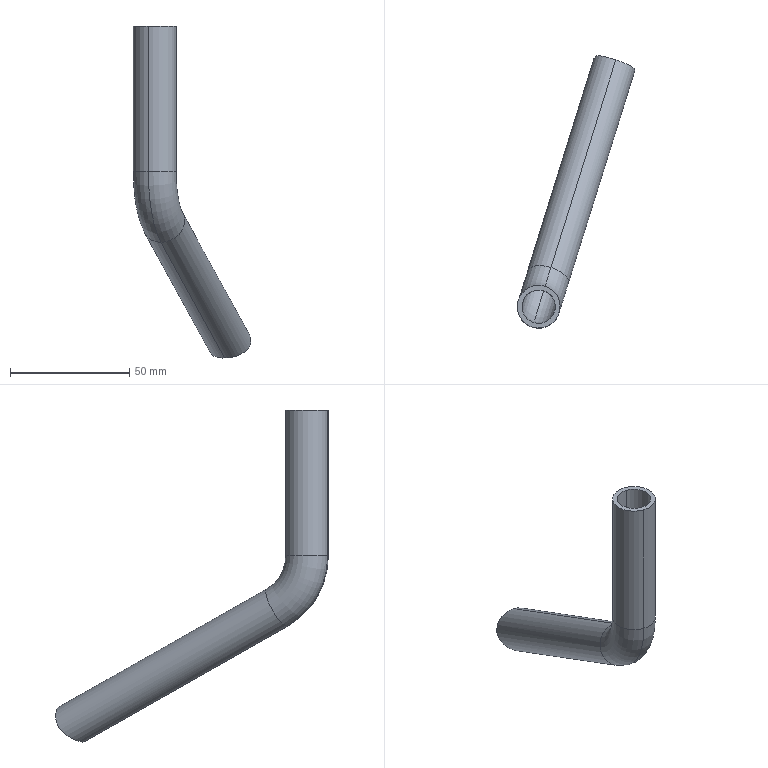Part | SolidWorks | features BaseBody 1 | 1 solid | 17 faces | box 49.357 x 114.676 x 139.496 mm | volume 19339 mm3 | cylinder 8 | spline 4 | torus 4 | plane 1 | commonest cylinder face diameters 14 x4 18 x4
STEP:
#1=CARTESIAN_POINT('',(32.452,94.694,-127.45));
#2=VERTEX_POINT('',#1);
#3=CARTESIAN_POINT('',(32.101,102.969,-116.416));
#4=VERTEX_POINT('',#3);
#5=CARTESIAN_POINT('',(32.452,94.694,-127.45));
#6=CARTESIAN_POINT('',(32.716,94.736,-127.396));
#7=CARTESIAN_POINT('',(33.249,94.856,-127.273));
#8=CARTESIAN_POINT('',(34.046,95.146,-127.049));
#9=CARTESIAN_POINT('',(34.836,95.548,-126.779));
#10=CARTESIAN_POINT('',(35.597,96.049,-126.464));
#11=CARTESIAN_POINT('',(36.325,96.649,-126.09));
#12=CARTESIAN_POINT('',(36.956,97.286,-125.671));
#13=CARTESIAN_POINT('',(37.437,97.864,-125.25));
#14=CARTESIAN_POINT('',(37.805,98.383,-124.818));
#15=CARTESIAN_POINT('',(38.075,98.836,-124.376));
#16=CARTESIAN_POINT('',(38.261,99.224,-123.927));
#17=CARTESIAN_POINT('',(38.377,99.559,-123.464));
#18=CARTESIAN_POINT('',(38.433,99.854,-122.972));
#19=CARTESIAN_POINT('',(38.426,100.121,-122.437));
#20=CARTESIAN_POINT('',(38.349,100.367,-121.842));
#21=CARTESIAN_POINT('',(38.186,100.594,-121.183));
#22=CARTESIAN_POINT('',(37.924,100.807,-120.472));
#23=CARTESIAN_POINT('',(37.548,101.015,-119.722));
#24=CARTESIAN_POINT('',(37.048,101.229,-118.965));
#25=CARTESIAN_POINT('',(36.455,101.448,-118.273));
#26=CARTESIAN_POINT('',(35.795,101.677,-117.678));
#27=CARTESIAN_POINT('',(35.106,101.913,-117.204));
#28=CARTESIAN_POINT('',(34.377,102.163,-116.834));
#29=CARTESIAN_POINT('',(33.621,102.427,-116.575));
#30=CARTESIAN_POINT('',(32.859,102.697,-116.432));
#31=CARTESIAN_POINT('',(32.352,102.878,-116.409));
#32=CARTESIAN_POINT('',(32.101,102.969,-116.416));
#33=B_SPLINE_CURVE_WITH_KNOTS('',3,(#5,#6,#7,#8,#9,#10,#11,#12,#13,#14,#15,#16,#17,#18,#19,#20,#21,#22,#23,#24,#25,#26,#27,#28,#29,#30,#31,#32),.UNSPECIFIED.,.F.,.F.,(4,1,1,1,1,1,1,1,1,1,1,1,1,1,1,1,1,1,1,1,1,1,1,1,1,4),(0.,0.04,0.08,0.12,0.16,0.2,0.24,0.28,0.32,0.36,0.4,0.44,0.48,0.52,0.56,0.6,0.64,0.68,0.72,0.76,0.8,0.84,0.88,0.92,0.96,1.),.UNSPECIFIED.);
#34=EDGE_CURVE('',#2,#4,#33,.T.);
#35=ORIENTED_EDGE('',*,*,#34,.F.);
#36=CARTESIAN_POINT('',(29.565,94.835,-127.721));
#37=VERTEX_POINT('',#36);
#38=CARTESIAN_POINT('',(29.565,94.835,-127.721));
#39=CARTESIAN_POINT('',(29.743,94.761,-127.712));
#40=CARTESIAN_POINT('',(30.105,94.639,-127.689));
#41=CARTESIAN_POINT('',(30.66,94.532,-127.645));
#42=CARTESIAN_POINT('',(31.232,94.5,-127.59));
#43=CARTESIAN_POINT('',(31.828,94.546,-127.526));
#44=CARTESIAN_POINT('',(32.242,94.635,-127.477));
#45=CARTESIAN_POINT('',(32.452,94.694,-127.45));
#46=B_SPLINE_CURVE_WITH_KNOTS('',3,(#38,#39,#40,#41,#42,#43,#44,#45),.UNSPECIFIED.,.F.,.F.,(4,1,1,1,1,4),(0.,0.2,0.4,0.6,0.8,1.),.UNSPECIFIED.);
#47=EDGE_CURVE('',#37,#2,#46,.T.);
#48=ORIENTED_EDGE('',*,*,#47,.F.);
#49=CARTESIAN_POINT('',(2.9,9.302,-79.129));
#50=VERTEX_POINT('',#49);
#51=CARTESIAN_POINT('',(29.565,94.835,-127.721));
#52=DIRECTION('',(-0.2616,-0.8392,0.4768));
#53=VECTOR('',#52,1000.);
#54=LINE('',#51,#53);
#55=EDGE_CURVE('',#37,#50,#54,.T.);
#56=ORIENTED_EDGE('',*,*,#55,.T.);
#57=CARTESIAN_POINT('',(4.887,15.674,-66.823));
#58=VERTEX_POINT('',#57);
#59=CARTESIAN_POINT('',(3.893,12.488,-72.976));
#60=DIRECTION('',(-0.2616,-0.8392,0.4768));
#61=DIRECTION('',(-0.1419,-0.4552,-0.879));
#62=AXIS2_PLACEMENT_3D('',#59,#60,#61);
#63=CIRCLE('',#62,7.);
#64=EDGE_CURVE('',#50,#58,#63,.T.);
#65=ORIENTED_EDGE('',*,*,#64,.T.);
#66=CARTESIAN_POINT('',(32.101,102.969,-116.416));
#67=DIRECTION('',(-0.2616,-0.8392,0.4768));
#68=VECTOR('',#67,1000.);
#69=LINE('',#66,#68);
#70=EDGE_CURVE('',#4,#58,#69,.T.);
#71=ORIENTED_EDGE('',*,*,#70,.F.);
#72=EDGE_LOOP('',(#35,#48,#56,#65,#71));
#73=FACE_OUTER_BOUND('',#72,.T.);
#74=CARTESIAN_POINT('',(3.893,12.488,-72.976));
#75=DIRECTION('',(0.2616,0.8392,-0.4768));
#76=DIRECTION('',(-0.1419,-0.4552,-0.879));
#77=AXIS2_PLACEMENT_3D('',#74,#75,#76);
#78=CYLINDRICAL_SURFACE('',#77,7.);
#79=ADVANCED_FACE('',(#73),#78,.F.);
#80=CARTESIAN_POINT('',(3.893,12.488,-72.976));
#81=DIRECTION('',(-0.2616,-0.8392,0.4768));
#82=DIRECTION('',(0.1419,0.4552,0.879));
#83=AXIS2_PLACEMENT_3D('',#80,#81,#82);
#84=CIRCLE('',#83,7.);
#85=EDGE_CURVE('',#58,#50,#84,.T.);
#86=ORIENTED_EDGE('',*,*,#85,.T.);
#87=ORIENTED_EDGE('',*,*,#55,.F.);
#88=CARTESIAN_POINT('',(28.332,95.591,-127.753));
#89=VERTEX_POINT('',#88);
#90=CARTESIAN_POINT('',(28.332,95.591,-127.753));
#91=CARTESIAN_POINT('',(28.466,95.48,-127.754));
#92=CARTESIAN_POINT('',(28.736,95.275,-127.752));
#93=CARTESIAN_POINT('',(29.146,95.025,-127.741));
#94=CARTESIAN_POINT('',(29.425,94.892,-127.728));
#95=CARTESIAN_POINT('',(29.565,94.835,-127.721));
#96=B_SPLINE_CURVE_WITH_KNOTS('',3,(#90,#91,#92,#93,#94,#95),.UNSPECIFIED.,.F.,.F.,(4,1,1,4),(0.,0.3333,0.6667,1.),.UNSPECIFIED.);
#97=EDGE_CURVE('',#89,#37,#96,.T.);
#98=ORIENTED_EDGE('',*,*,#97,.F.);
#99=CARTESIAN_POINT('',(32.101,102.969,-116.416));
#100=CARTESIAN_POINT('',(31.841,103.063,-116.422));
#101=CARTESIAN_POINT('',(31.316,103.253,-116.473));
#102=CARTESIAN_POINT('',(30.528,103.538,-116.666));
#103=CARTESIAN_POINT('',(29.741,103.819,-116.98));
#104=CARTESIAN_POINT('',(28.969,104.086,-117.417));
#105=CARTESIAN_POINT('',(28.225,104.325,-117.976));
#106=CARTESIAN_POINT('',(27.53,104.518,-118.642));
#107=CARTESIAN_POINT('',(26.912,104.645,-119.38));
#108=CARTESIAN_POINT('',(26.375,104.69,-120.163));
#109=CARTESIAN_POINT('',(25.935,104.643,-120.94));
#110=CARTESIAN_POINT('',(25.586,104.506,-121.677));
#111=CARTESIAN_POINT('',(25.315,104.284,-122.364));
#112=CARTESIAN_POINT('',(25.108,103.984,-122.996));
#113=CARTESIAN_POINT('',(24.955,103.607,-123.586));
#114=CARTESIAN_POINT('',(24.849,103.132,-124.163));
#115=CARTESIAN_POINT('',(24.798,102.534,-124.735));
#116=CARTESIAN_POINT('',(24.818,101.826,-125.28));
#117=CARTESIAN_POINT('',(24.925,101.001,-125.805));
#118=CARTESIAN_POINT('',(25.148,100.063,-126.3));
#119=CARTESIAN_POINT('',(25.484,99.12,-126.721));
#120=CARTESIAN_POINT('',(25.921,98.22,-127.066));
#121=CARTESIAN_POINT('',(26.447,97.394,-127.338));
#122=CARTESIAN_POINT('',(27.032,96.678,-127.537));
#123=CARTESIAN_POINT('',(27.665,96.069,-127.676));
#124=CARTESIAN_POINT('',(28.108,95.738,-127.732));
#125=CARTESIAN_POINT('',(28.332,95.591,-127.753));
#126=B_SPLINE_CURVE_WITH_KNOTS('',3,(#99,#100,#101,#102,#103,#104,#105,#106,#107,#108,#109,#110,#111,#112,#113,#114,#115,#116,#117,#118,#119,#120,#121,#122,#123,#124,#125),.UNSPECIFIED.,.F.,.F.,(4,1,1,1,1,1,1,1,1,1,1,1,1,1,1,1,1,1,1,1,1,1,1,1,4),(0.,0.04167,0.08333,0.125,0.1667,0.2083,0.25,0.2917,0.3333,0.375,0.4167,0.4583,0.5,0.5417,0.5833,0.625,0.6667,0.7083,0.75,0.7917,0.8333,0.875,0.9167,0.9583,1.),.UNSPECIFIED.);
#127=EDGE_CURVE('',#4,#89,#126,.T.);
#128=ORIENTED_EDGE('',*,*,#127,.F.);
#129=ORIENTED_EDGE('',*,*,#70,.T.);
#130=EDGE_LOOP('',(#86,#87,#98,#128,#129));
#131=FACE_OUTER_BOUND('',#130,.T.);
#132=CARTESIAN_POINT('',(3.893,12.488,-72.976));
#133=DIRECTION('',(0.2616,0.8392,-0.4768));
#134=DIRECTION('',(-0.1419,-0.4552,-0.879));
#135=AXIS2_PLACEMENT_3D('',#132,#133,#134);
#136=CYLINDRICAL_SURFACE('',#135,7.);
#137=ADVANCED_FACE('',(#131),#136,.F.);
#138=CARTESIAN_POINT('',(27.672,94.819,-129.475));
#139=VERTEX_POINT('',#138);
#140=CARTESIAN_POINT('',(27.672,94.819,-129.475));
#141=DIRECTION('',(0.3303,0.3863,0.8612));
#142=VECTOR('',#141,1000.);
#143=LINE('',#140,#142);
#144=EDGE_CURVE('',#139,#89,#143,.T.);
#145=ORIENTED_EDGE('',*,*,#144,.F.);
#146=CARTESIAN_POINT('',(32.385,103.879,-114.658));
#147=VERTEX_POINT('',#146);
#148=CARTESIAN_POINT('',(27.672,94.819,-129.475));
#149=CARTESIAN_POINT('',(27.379,94.995,-129.442));
#150=CARTESIAN_POINT('',(26.799,95.388,-129.351));
#151=CARTESIAN_POINT('',(25.964,96.103,-129.135));
#152=CARTESIAN_POINT('',(25.186,96.939,-128.83));
#153=CARTESIAN_POINT('',(24.478,97.9,-128.422));
#154=CARTESIAN_POINT('',(23.881,98.942,-127.914));
#155=CARTESIAN_POINT('',(23.411,100.034,-127.304));
#156=CARTESIAN_POINT('',(23.087,101.122,-126.6));
#157=CARTESIAN_POINT('',(22.919,102.084,-125.87));
#158=CARTESIAN_POINT('',(22.869,102.915,-125.124));
#159=CARTESIAN_POINT('',(22.916,103.625,-124.355));
#160=CARTESIAN_POINT('',(23.042,104.2,-123.592));
#161=CARTESIAN_POINT('',(23.232,104.667,-122.823));
#162=CARTESIAN_POINT('',(23.498,105.051,-122.01));
#163=CARTESIAN_POINT('',(23.852,105.353,-121.137));
#164=CARTESIAN_POINT('',(24.311,105.564,-120.21));
#165=CARTESIAN_POINT('',(24.894,105.677,-119.239));
#166=CARTESIAN_POINT('',(25.604,105.683,-118.269));
#167=CARTESIAN_POINT('',(26.421,105.592,-117.361));
#168=CARTESIAN_POINT('',(27.336,105.415,-116.545));
#169=CARTESIAN_POINT('',(28.313,105.172,-115.864));
#170=CARTESIAN_POINT('',(29.323,104.885,-115.334));
#171=CARTESIAN_POINT('',(30.348,104.567,-114.955));
#172=CARTESIAN_POINT('',(31.371,104.229,-114.723));
#173=CARTESIAN_POINT('',(32.05,103.996,-114.664));
#174=CARTESIAN_POINT('',(32.385,103.879,-114.658));
#175=B_SPLINE_CURVE_WITH_KNOTS('',3,(#148,#149,#150,#151,#152,#153,#154,#155,#156,#157,#158,#159,#160,#161,#162,#163,#164,#165,#166,#167,#168,#169,#170,#171,#172,#173,#174),.UNSPECIFIED.,.F.,.F.,(4,1,1,1,1,1,1,1,1,1,1,1,1,1,1,1,1,1,1,1,1,1,1,1,4),(0.,0.04167,0.08333,0.125,0.1667,0.2083,0.25,0.2917,0.3333,0.375,0.4167,0.4583,0.5,0.5417,0.5833,0.625,0.6667,0.7083,0.75,0.7917,0.8333,0.875,0.9167,0.9583,1.),.UNSPECIFIED.);
#176=EDGE_CURVE('',#139,#147,#175,.T.);
#177=ORIENTED_EDGE('',*,*,#176,.T.);
#178=CARTESIAN_POINT('',(32.385,103.879,-114.658));
#179=DIRECTION('',(-0.1419,-0.4552,-0.879));
#180=VECTOR('',#179,1000.);
#181=LINE('',#178,#180);
#182=EDGE_CURVE('',#147,#4,#181,.T.);
#183=ORIENTED_EDGE('',*,*,#182,.T.);
#184=ORIENTED_EDGE('',*,*,#127,.T.);
#185=EDGE_LOOP('',(#145,#177,#183,#184));
#186=FACE_OUTER_BOUND('',#185,.T.);
#187=CARTESIAN_POINT('',(28.549,95.525,-127.663));
#188=CARTESIAN_POINT('',(28.323,95.228,-128.31));
#189=CARTESIAN_POINT('',(28.097,94.931,-128.956));
#190=CARTESIAN_POINT('',(27.871,94.635,-129.603));
#191=CARTESIAN_POINT('',(28.49,95.561,-127.659));
#192=CARTESIAN_POINT('',(28.257,95.267,-128.304));
#193=CARTESIAN_POINT('',(28.024,94.973,-128.95));
#194=CARTESIAN_POINT('',(27.791,94.679,-129.596));
#195=CARTESIAN_POINT('',(28.21,95.739,-127.637));
#196=CARTESIAN_POINT('',(27.945,95.459,-128.277));
#197=CARTESIAN_POINT('',(27.679,95.178,-128.917));
#198=CARTESIAN_POINT('',(27.414,94.897,-129.557));
#199=CARTESIAN_POINT('',(27.717,96.11,-127.576));
#200=CARTESIAN_POINT('',(27.393,95.856,-128.201));
#201=CARTESIAN_POINT('',(27.07,95.601,-128.826));
#202=CARTESIAN_POINT('',(26.747,95.347,-129.452));
#203=CARTESIAN_POINT('',(27.096,96.712,-127.442));
#204=CARTESIAN_POINT('',(26.697,96.498,-128.038));
#205=CARTESIAN_POINT('',(26.299,96.283,-128.634));
#206=CARTESIAN_POINT('',(25.9,96.069,-129.23));
#207=CARTESIAN_POINT('',(26.523,97.421,-127.248));
#208=CARTESIAN_POINT('',(26.052,97.251,-127.805));
#209=CARTESIAN_POINT('',(25.581,97.082,-128.362));
#210=CARTESIAN_POINT('',(25.11,96.912,-128.919));
#211=CARTESIAN_POINT('',(26.008,98.24,-126.984));
#212=CARTESIAN_POINT('',(25.469,98.12,-127.491));
#213=CARTESIAN_POINT('',(24.93,98.,-127.997));
#214=CARTESIAN_POINT('',(24.392,97.88,-128.503));
#215=CARTESIAN_POINT('',(25.581,99.131,-126.649));
#216=CARTESIAN_POINT('',(24.982,99.064,-127.095));
#217=CARTESIAN_POINT('',(24.384,98.998,-127.54));
#218=CARTESIAN_POINT('',(23.785,98.931,-127.986));
#219=CARTESIAN_POINT('',(25.252,100.065,-126.24));
#220=CARTESIAN_POINT('',(24.604,100.054,-126.615));
#221=CARTESIAN_POINT('',(23.955,100.043,-126.99));
#222=CARTESIAN_POINT('',(23.307,100.032,-127.365));
#223=CARTESIAN_POINT('',(25.035,100.994,-125.757));
#224=CARTESIAN_POINT('',(24.349,101.039,-126.054));
#225=CARTESIAN_POINT('',(23.663,101.084,-126.351));
#226=CARTESIAN_POINT('',(22.977,101.129,-126.648));
#227=CARTESIAN_POINT('',(24.932,101.811,-125.245));
#228=CARTESIAN_POINT('',(24.223,101.907,-125.465));
#229=CARTESIAN_POINT('',(23.514,102.003,-125.685));
#230=CARTESIAN_POINT('',(22.805,102.099,-125.905));
#231=CARTESIAN_POINT('',(24.914,102.511,-124.712));
#232=CARTESIAN_POINT('',(24.194,102.653,-124.857));
#233=CARTESIAN_POINT('',(23.473,102.795,-125.002));
#234=CARTESIAN_POINT('',(22.753,102.937,-125.147));
#235=CARTESIAN_POINT('',(24.965,103.102,-124.151));
#236=CARTESIAN_POINT('',(24.244,103.286,-124.223));
#237=CARTESIAN_POINT('',(23.522,103.471,-124.295));
#238=CARTESIAN_POINT('',(22.8,103.655,-124.366));
#239=CARTESIAN_POINT('',(25.07,103.572,-123.585));
#240=CARTESIAN_POINT('',(24.356,103.793,-123.588));
#241=CARTESIAN_POINT('',(23.641,104.014,-123.59));
#242=CARTESIAN_POINT('',(22.927,104.236,-123.593));
#243=CARTESIAN_POINT('',(25.221,103.943,-123.006));
#244=CARTESIAN_POINT('',(24.52,104.198,-122.942));
#245=CARTESIAN_POINT('',(23.82,104.453,-122.877));
#246=CARTESIAN_POINT('',(23.12,104.708,-122.813));
#247=CARTESIAN_POINT('',(25.424,104.238,-122.385));
#248=CARTESIAN_POINT('',(24.745,104.524,-122.253));
#249=CARTESIAN_POINT('',(24.067,104.811,-122.121));
#250=CARTESIAN_POINT('',(23.388,105.097,-121.989));
#251=CARTESIAN_POINT('',(25.69,104.455,-121.71));
#252=CARTESIAN_POINT('',(25.043,104.771,-121.508));
#253=CARTESIAN_POINT('',(24.396,105.088,-121.307));
#254=CARTESIAN_POINT('',(23.748,105.404,-121.105));
#255=CARTESIAN_POINT('',(26.033,104.588,-120.984));
#256=CARTESIAN_POINT('',(25.426,104.932,-120.712));
#257=CARTESIAN_POINT('',(24.82,105.276,-120.439));
#258=CARTESIAN_POINT('',(24.214,105.62,-120.166));
#259=CARTESIAN_POINT('',(26.465,104.631,-120.218));
#260=CARTESIAN_POINT('',(25.911,104.999,-119.873));
#261=CARTESIAN_POINT('',(25.358,105.367,-119.529));
#262=CARTESIAN_POINT('',(24.805,105.736,-119.184));
#263=CARTESIAN_POINT('',(26.99,104.582,-119.446));
#264=CARTESIAN_POINT('',(26.502,104.97,-119.032));
#265=CARTESIAN_POINT('',(26.014,105.358,-118.617));
#266=CARTESIAN_POINT('',(25.525,105.746,-118.203));
#267=CARTESIAN_POINT('',(27.597,104.454,-118.719));
#268=CARTESIAN_POINT('',(27.183,104.854,-118.24));
#269=CARTESIAN_POINT('',(26.769,105.255,-117.762));
#270=CARTESIAN_POINT('',(26.354,105.656,-117.284));
#271=CARTESIAN_POINT('',(28.278,104.26,-118.062));
#272=CARTESIAN_POINT('',(27.946,104.666,-117.528));
#273=CARTESIAN_POINT('',(27.614,105.073,-116.994));
#274=CARTESIAN_POINT('',(27.283,105.48,-116.46));
#275=CARTESIAN_POINT('',(29.008,104.02,-117.511));
#276=CARTESIAN_POINT('',(28.764,104.426,-116.931));
#277=CARTESIAN_POINT('',(28.519,104.832,-116.351));
#278=CARTESIAN_POINT('',(28.274,105.238,-115.771));
#279=CARTESIAN_POINT('',(29.766,103.755,-117.079));
#280=CARTESIAN_POINT('',(29.61,104.153,-116.465));
#281=CARTESIAN_POINT('',(29.454,104.551,-115.85));
#282=CARTESIAN_POINT('',(29.298,104.949,-115.235));
#283=CARTESIAN_POINT('',(30.538,103.476,-116.769));
#284=CARTESIAN_POINT('',(30.471,103.86,-116.13));
#285=CARTESIAN_POINT('',(30.404,104.244,-115.491));
#286=CARTESIAN_POINT('',(30.337,104.628,-114.852));
#287=CARTESIAN_POINT('',(31.313,103.194,-116.578));
#288=CARTESIAN_POINT('',(31.334,103.559,-115.925));
#289=CARTESIAN_POINT('',(31.354,103.923,-115.272));
#290=CARTESIAN_POINT('',(31.375,104.288,-114.618));
#291=CARTESIAN_POINT('',(31.895,102.982,-116.521));
#292=CARTESIAN_POINT('',(31.98,103.329,-115.865));
#293=CARTESIAN_POINT('',(32.065,103.676,-115.208));
#294=CARTESIAN_POINT('',(32.15,104.022,-114.551));
#295=CARTESIAN_POINT('',(32.215,102.867,-116.519));
#296=CARTESIAN_POINT('',(32.335,103.202,-115.863));
#297=CARTESIAN_POINT('',(32.455,103.538,-115.207));
#298=CARTESIAN_POINT('',(32.575,103.873,-114.55));
#299=CARTESIAN_POINT('',(32.28,102.844,-116.52));
#300=CARTESIAN_POINT('',(32.407,103.177,-115.864));
#301=CARTESIAN_POINT('',(32.534,103.51,-115.208));
#302=CARTESIAN_POINT('',(32.662,103.843,-114.552));
#303=B_SPLINE_SURFACE_WITH_KNOTS('',3,3,((#187,#188,#189,#190),(#191,#192,#193,#194),(#195,#196,#197,#198),(#199,#200,#201,#202),(#203,#204,#205,#206),(#207,#208,#209,#210),(#211,#212,#213,#214),(#215,#216,#217,#218),(#219,#220,#221,#222),(#223,#224,#225,#226),(#227,#228,#229,#230),(#231,#232,#233,#234),(#235,#236,#237,#238),(#239,#240,#241,#242),(#243,#244,#245,#246),(#247,#248,#249,#250),(#251,#252,#253,#254),(#255,#256,#257,#258),(#259,#260,#261,#262),(#263,#264,#265,#266),(#267,#268,#269,#270),(#271,#272,#273,#274),(#275,#276,#277,#278),(#279,#280,#281,#282),(#283,#284,#285,#286),(#287,#288,#289,#290),(#291,#292,#293,#294),(#295,#296,#297,#298),(#299,#300,#301,#302)),.UNSPECIFIED.,.F.,.F.,.F.,(4,1,1,1,1,1,1,1,1,1,1,1,1,1,1,1,1,1,1,1,1,1,1,1,1,1,4),(4,4),(-0.01113,0.,0.04167,0.08333,0.125,0.1667,0.2083,0.25,0.2917,0.3333,0.375,0.4167,0.4583,0.5,0.5417,0.5833,0.625,0.6667,0.7083,0.75,0.7917,0.8333,0.875,0.9167,0.9583,1.,1.011),(-0.06007,1.06),.UNSPECIFIED.);
#304=ADVANCED_FACE('',(#186),#303,.F.);
#305=ORIENTED_EDGE('',*,*,#182,.F.);
#306=CARTESIAN_POINT('',(32.955,93.621,-129.062));
#307=VERTEX_POINT('',#306);
#308=CARTESIAN_POINT('',(32.385,103.879,-114.658));
#309=CARTESIAN_POINT('',(32.709,103.766,-114.651));
#310=CARTESIAN_POINT('',(33.361,103.534,-114.681));
#311=CARTESIAN_POINT('',(34.338,103.178,-114.86));
#312=CARTESIAN_POINT('',(35.303,102.815,-115.179));
#313=CARTESIAN_POINT('',(36.228,102.455,-115.633));
#314=CARTESIAN_POINT('',(37.098,102.103,-116.214));
#315=CARTESIAN_POINT('',(37.927,101.744,-116.944));
#316=CARTESIAN_POINT('',(38.667,101.39,-117.793));
#317=CARTESIAN_POINT('',(39.286,101.041,-118.723));
#318=CARTESIAN_POINT('',(39.748,100.706,-119.649));
#319=CARTESIAN_POINT('',(40.069,100.377,-120.532));
#320=CARTESIAN_POINT('',(40.266,100.045,-121.357));
#321=CARTESIAN_POINT('',(40.357,99.706,-122.108));
#322=CARTESIAN_POINT('',(40.363,99.355,-122.792));
#323=CARTESIAN_POINT('',(40.294,98.981,-123.429));
#324=CARTESIAN_POINT('',(40.151,98.573,-124.036));
#325=CARTESIAN_POINT('',(39.924,98.112,-124.635));
#326=CARTESIAN_POINT('',(39.595,97.587,-125.236));
#327=CARTESIAN_POINT('',(39.146,96.998,-125.836));
#328=CARTESIAN_POINT('',(38.558,96.354,-126.433));
#329=CARTESIAN_POINT('',(37.784,95.655,-127.04));
#330=CARTESIAN_POINT('',(36.887,95.007,-127.591));
#331=CARTESIAN_POINT('',(35.944,94.475,-128.06));
#332=CARTESIAN_POINT('',(34.959,94.058,-128.463));
#333=CARTESIAN_POINT('',(33.961,93.768,-128.798));
#334=CARTESIAN_POINT('',(33.289,93.656,-128.981));
#335=CARTESIAN_POINT('',(32.955,93.621,-129.062));
#336=B_SPLINE_CURVE_WITH_KNOTS('',3,(#308,#309,#310,#311,#312,#313,#314,#315,#316,#317,#318,#319,#320,#321,#322,#323,#324,#325,#326,#327,#328,#329,#330,#331,#332,#333,#334,#335),.UNSPECIFIED.,.F.,.F.,(4,1,1,1,1,1,1,1,1,1,1,1,1,1,1,1,1,1,1,1,1,1,1,1,1,4),(0.,0.04,0.08,0.12,0.16,0.2,0.24,0.28,0.32,0.36,0.4,0.44,0.48,0.52,0.56,0.6,0.64,0.68,0.72,0.76,0.8,0.84,0.88,0.92,0.96,1.),.UNSPECIFIED.);
#337=EDGE_CURVE('',#147,#307,#336,.T.);
#338=ORIENTED_EDGE('',*,*,#337,.T.);
#339=CARTESIAN_POINT('',(32.955,93.621,-129.062));
#340=DIRECTION('',(-0.2515,0.5362,0.8058));
#341=VECTOR('',#340,1000.);
#342=LINE('',#339,#341);
#343=EDGE_CURVE('',#307,#2,#342,.T.);
#344=ORIENTED_EDGE('',*,*,#343,.T.);
#345=ORIENTED_EDGE('',*,*,#34,.T.);
#346=EDGE_LOOP('',(#305,#338,#344,#345));
#347=FACE_OUTER_BOUND('',#346,.T.);
#348=CARTESIAN_POINT('',(31.901,102.98,-116.529));
#349=CARTESIAN_POINT('',(31.987,103.326,-115.873));
#350=CARTESIAN_POINT('',(32.073,103.672,-115.217));
#351=CARTESIAN_POINT('',(32.158,104.018,-114.561));
#352=CARTESIAN_POINT('',(31.962,102.958,-116.526));
#353=CARTESIAN_POINT('',(32.054,103.302,-115.869));
#354=CARTESIAN_POINT('',(32.147,103.646,-115.213));
#355=CARTESIAN_POINT('',(32.239,103.99,-114.557));
#356=CARTESIAN_POINT('',(32.269,102.847,-116.512));
#357=CARTESIAN_POINT('',(32.396,103.181,-115.856));
#358=CARTESIAN_POINT('',(32.522,103.515,-115.199));
#359=CARTESIAN_POINT('',(32.648,103.848,-114.542));
#360=CARTESIAN_POINT('',(32.829,102.646,-116.537));
#361=CARTESIAN_POINT('',(33.016,102.959,-115.883));
#362=CARTESIAN_POINT('',(33.204,103.272,-115.23));
#363=CARTESIAN_POINT('',(33.391,103.585,-114.576));
#364=CARTESIAN_POINT('',(33.578,102.382,-116.679));
#365=CARTESIAN_POINT('',(33.846,102.662,-116.038));
#366=CARTESIAN_POINT('',(34.113,102.942,-115.398));
#367=CARTESIAN_POINT('',(34.381,103.223,-114.758));
#368=CARTESIAN_POINT('',(34.322,102.124,-116.933));
#369=CARTESIAN_POINT('',(34.667,102.367,-116.315));
#370=CARTESIAN_POINT('',(35.013,102.611,-115.697));
#371=CARTESIAN_POINT('',(35.358,102.854,-115.08));
#372=CARTESIAN_POINT('',(35.039,101.88,-117.298));
#373=CARTESIAN_POINT('',(35.458,102.083,-116.712));
#374=CARTESIAN_POINT('',(35.877,102.285,-116.125));
#375=CARTESIAN_POINT('',(36.295,102.488,-115.539));
#376=CARTESIAN_POINT('',(35.717,101.652,-117.766));
#377=CARTESIAN_POINT('',(36.203,101.811,-117.219));
#378=CARTESIAN_POINT('',(36.69,101.969,-116.673));
#379=CARTESIAN_POINT('',(37.176,102.128,-116.126));
#380=CARTESIAN_POINT('',(36.367,101.43,-118.353));
#381=CARTESIAN_POINT('',(36.917,101.541,-117.857));
#382=CARTESIAN_POINT('',(37.466,101.651,-117.36));
#383=CARTESIAN_POINT('',(38.016,101.762,-116.864));
#384=CARTESIAN_POINT('',(36.951,101.219,-119.036));
#385=CARTESIAN_POINT('',(37.556,101.279,-118.598));
#386=CARTESIAN_POINT('',(38.16,101.339,-118.16));
#387=CARTESIAN_POINT('',(38.764,101.4,-117.723));
#388=CARTESIAN_POINT('',(37.443,101.014,-119.782));
#389=CARTESIAN_POINT('',(38.092,101.023,-119.409));
#390=CARTESIAN_POINT('',(38.741,101.033,-119.036));
#391=CARTESIAN_POINT('',(39.39,101.043,-118.663));
#392=CARTESIAN_POINT('',(37.814,100.813,-120.521));
#393=CARTESIAN_POINT('',(38.496,100.775,-120.214));
#394=CARTESIAN_POINT('',(39.177,100.738,-119.907));
#395=CARTESIAN_POINT('',(39.858,100.7,-119.599));
#396=CARTESIAN_POINT('',(38.073,100.607,-121.222));
#397=CARTESIAN_POINT('',(38.776,100.526,-120.979));
#398=CARTESIAN_POINT('',(39.479,100.445,-120.736));
#399=CARTESIAN_POINT('',(40.182,100.364,-120.493));
#400=CARTESIAN_POINT('',(38.234,100.386,-121.871));
#401=CARTESIAN_POINT('',(38.949,100.266,-121.69));
#402=CARTESIAN_POINT('',(39.665,100.146,-121.509));
#403=CARTESIAN_POINT('',(40.381,100.026,-121.327));
#404=CARTESIAN_POINT('',(38.31,100.146,-122.457));
#405=CARTESIAN_POINT('',(39.031,99.991,-122.334));
#406=CARTESIAN_POINT('',(39.752,99.836,-122.211));
#407=CARTESIAN_POINT('',(40.473,99.681,-122.088));
#408=CARTESIAN_POINT('',(38.317,99.884,-122.983));
#409=CARTESIAN_POINT('',(39.037,99.698,-122.916));
#410=CARTESIAN_POINT('',(39.758,99.511,-122.849));
#411=CARTESIAN_POINT('',(40.479,99.325,-122.782));
#412=CARTESIAN_POINT('',(38.262,99.593,-123.466));
#413=CARTESIAN_POINT('',(38.978,99.378,-123.453));
#414=CARTESIAN_POINT('',(39.693,99.162,-123.44));
#415=CARTESIAN_POINT('',(40.409,98.947,-123.426));
#416=CARTESIAN_POINT('',(38.147,99.263,-123.92));
#417=CARTESIAN_POINT('',(38.853,99.02,-123.961));
#418=CARTESIAN_POINT('',(39.559,98.777,-124.002));
#419=CARTESIAN_POINT('',(40.265,98.534,-124.042));
#420=CARTESIAN_POINT('',(37.964,98.88,-124.361));
#421=CARTESIAN_POINT('',(38.654,98.609,-124.458));
#422=CARTESIAN_POINT('',(39.345,98.339,-124.554));
#423=CARTESIAN_POINT('',(40.035,98.069,-124.651));
#424=CARTESIAN_POINT('',(37.698,98.431,-124.793));
#425=CARTESIAN_POINT('',(38.366,98.134,-124.949));
#426=CARTESIAN_POINT('',(39.034,97.837,-125.105));
#427=CARTESIAN_POINT('',(39.703,97.54,-125.261));
#428=CARTESIAN_POINT('',(37.334,97.916,-125.215));
#429=CARTESIAN_POINT('',(37.972,97.593,-125.434));
#430=CARTESIAN_POINT('',(38.611,97.27,-125.652));
#431=CARTESIAN_POINT('',(39.249,96.946,-125.871));
#432=CARTESIAN_POINT('',(36.86,97.342,-125.625));
#433=CARTESIAN_POINT('',(37.458,96.994,-125.91));
#434=CARTESIAN_POINT('',(38.056,96.646,-126.194));
#435=CARTESIAN_POINT('',(38.654,96.298,-126.479));
#436=CARTESIAN_POINT('',(36.237,96.709,-126.033));
#437=CARTESIAN_POINT('',(36.782,96.338,-126.387));
#438=CARTESIAN_POINT('',(37.327,95.967,-126.742));
#439=CARTESIAN_POINT('',(37.872,95.595,-127.096));
#440=CARTESIAN_POINT('',(35.519,96.112,-126.396));
#441=CARTESIAN_POINT('',(36.001,95.723,-126.817));
#442=CARTESIAN_POINT('',(36.482,95.334,-127.238));
#443=CARTESIAN_POINT('',(36.964,94.945,-127.658));
#444=CARTESIAN_POINT('',(34.77,95.613,-126.702));
#445=CARTESIAN_POINT('',(35.183,95.212,-127.18));
#446=CARTESIAN_POINT('',(35.597,94.811,-127.659));
#447=CARTESIAN_POINT('',(36.011,94.411,-128.137));
#448=CARTESIAN_POINT('',(33.991,95.212,-126.964));
#449=CARTESIAN_POINT('',(34.332,94.805,-127.492));
#450=CARTESIAN_POINT('',(34.673,94.399,-128.02));
#451=CARTESIAN_POINT('',(35.014,93.993,-128.548));
#452=CARTESIAN_POINT('',(33.207,94.922,-127.181));
#453=CARTESIAN_POINT('',(33.472,94.515,-127.751));
#454=CARTESIAN_POINT('',(33.738,94.109,-128.321));
#455=CARTESIAN_POINT('',(34.003,93.702,-128.89));
#456=CARTESIAN_POINT('',(32.618,94.786,-127.315));
#457=CARTESIAN_POINT('',(32.825,94.383,-127.91));
#458=CARTESIAN_POINT('',(33.033,93.981,-128.504));
#459=CARTESIAN_POINT('',(33.24,93.578,-129.099));
#460=CARTESIAN_POINT('',(32.294,94.738,-127.379));
#461=CARTESIAN_POINT('',(32.469,94.339,-127.986));
#462=CARTESIAN_POINT('',(32.644,93.94,-128.592));
#463=CARTESIAN_POINT('',(32.819,93.541,-129.199));
#464=CARTESIAN_POINT('',(32.231,94.73,-127.391));
#465=CARTESIAN_POINT('',(32.399,94.332,-128.));
#466=CARTESIAN_POINT('',(32.568,93.933,-128.609));
#467=CARTESIAN_POINT('',(32.737,93.535,-129.217));
#468=B_SPLINE_SURFACE_WITH_KNOTS('',3,3,((#348,#349,#350,#351),(#352,#353,#354,#355),(#356,#357,#358,#359),(#360,#361,#362,#363),(#364,#365,#366,#367),(#368,#369,#370,#371),(#372,#373,#374,#375),(#376,#377,#378,#379),(#380,#381,#382,#383),(#384,#385,#386,#387),(#388,#389,#390,#391),(#392,#393,#394,#395),(#396,#397,#398,#399),(#400,#401,#402,#403),(#404,#405,#406,#407),(#408,#409,#410,#411),(#412,#413,#414,#415),(#416,#417,#418,#419),(#420,#421,#422,#423),(#424,#425,#426,#427),(#428,#429,#430,#431),(#432,#433,#434,#435),(#436,#437,#438,#439),(#440,#441,#442,#443),(#444,#445,#446,#447),(#448,#449,#450,#451),(#452,#453,#454,#455),(#456,#457,#458,#459),(#460,#461,#462,#463),(#464,#465,#466,#467)),.UNSPECIFIED.,.F.,.F.,.F.,(4,1,1,1,1,1,1,1,1,1,1,1,1,1,1,1,1,1,1,1,1,1,1,1,1,1,1,4),(4,4),(-0.009922,0.,0.04,0.08,0.12,0.16,0.2,0.24,0.28,0.32,0.36,0.4,0.44,0.48,0.52,0.56,0.6,0.64,0.68,0.72,0.76,0.8,0.84,0.88,0.92,0.96,1.,1.01),(-0.06008,1.06),.UNSPECIFIED.);
#469=ADVANCED_FACE('',(#347),#468,.F.);
#470=ORIENTED_EDGE('',*,*,#343,.F.);
#471=CARTESIAN_POINT('',(29.282,93.924,-129.479));
#472=VERTEX_POINT('',#471);
#473=CARTESIAN_POINT('',(32.955,93.621,-129.062));
#474=CARTESIAN_POINT('',(32.692,93.568,-129.108));
#475=CARTESIAN_POINT('',(32.172,93.492,-129.193));
#476=CARTESIAN_POINT('',(31.417,93.472,-129.298));
#477=CARTESIAN_POINT('',(30.689,93.536,-129.381));
#478=CARTESIAN_POINT('',(29.978,93.682,-129.443));
#479=CARTESIAN_POINT('',(29.512,93.835,-129.47));
#480=CARTESIAN_POINT('',(29.282,93.924,-129.479));
#481=B_SPLINE_CURVE_WITH_KNOTS('',3,(#473,#474,#475,#476,#477,#478,#479,#480),.UNSPECIFIED.,.F.,.F.,(4,1,1,1,1,4),(0.,0.2,0.4,0.6,0.8,1.),.UNSPECIFIED.);
#482=EDGE_CURVE('',#307,#472,#481,.T.);
#483=ORIENTED_EDGE('',*,*,#482,.T.);
#484=CARTESIAN_POINT('',(29.282,93.924,-129.479));
#485=DIRECTION('',(0.1419,0.4552,0.879));
#486=VECTOR('',#485,1000.);
#487=LINE('',#484,#486);
#488=EDGE_CURVE('',#472,#37,#487,.T.);
#489=ORIENTED_EDGE('',*,*,#488,.T.);
#490=ORIENTED_EDGE('',*,*,#47,.T.);
#491=EDGE_LOOP('',(#470,#483,#489,#490));
#492=FACE_OUTER_BOUND('',#491,.T.);
#493=CARTESIAN_POINT('',(29.527,94.913,-127.619));
#494=CARTESIAN_POINT('',(29.415,94.575,-128.275));
#495=CARTESIAN_POINT('',(29.303,94.237,-128.931));
#496=CARTESIAN_POINT('',(29.191,93.899,-129.588));
#497=CARTESIAN_POINT('',(29.546,94.905,-127.618));
#498=CARTESIAN_POINT('',(29.436,94.566,-128.274));
#499=CARTESIAN_POINT('',(29.326,94.228,-128.93));
#500=CARTESIAN_POINT('',(29.216,93.889,-129.587));
#501=CARTESIAN_POINT('',(29.738,94.823,-127.608));
#502=CARTESIAN_POINT('',(29.65,94.478,-128.264));
#503=CARTESIAN_POINT('',(29.561,94.132,-128.92));
#504=CARTESIAN_POINT('',(29.473,93.787,-129.577));
#505=CARTESIAN_POINT('',(30.113,94.697,-127.584));
#506=CARTESIAN_POINT('',(30.065,94.339,-128.239));
#507=CARTESIAN_POINT('',(30.018,93.982,-128.894));
#508=CARTESIAN_POINT('',(29.971,93.625,-129.548));
#509=CARTESIAN_POINT('',(30.658,94.592,-127.54));
#510=CARTESIAN_POINT('',(30.669,94.22,-128.189));
#511=CARTESIAN_POINT('',(30.68,93.848,-128.837));
#512=CARTESIAN_POINT('',(30.69,93.476,-129.485));
#513=CARTESIAN_POINT('',(31.221,94.561,-127.488));
#514=CARTESIAN_POINT('',(31.29,94.178,-128.125));
#515=CARTESIAN_POINT('',(31.359,93.794,-128.763));
#516=CARTESIAN_POINT('',(31.429,93.41,-129.401));
#517=CARTESIAN_POINT('',(31.807,94.609,-127.426));
#518=CARTESIAN_POINT('',(31.936,94.216,-128.048));
#519=CARTESIAN_POINT('',(32.064,93.822,-128.671));
#520=CARTESIAN_POINT('',(32.192,93.429,-129.293));
#521=CARTESIAN_POINT('',(32.234,94.703,-127.377));
#522=CARTESIAN_POINT('',(32.404,94.304,-127.985));
#523=CARTESIAN_POINT('',(32.573,93.906,-128.594));
#524=CARTESIAN_POINT('',(32.743,93.507,-129.202));
#525=CARTESIAN_POINT('',(32.46,94.769,-127.349));
#526=CARTESIAN_POINT('',(32.652,94.368,-127.949));
#527=CARTESIAN_POINT('',(32.843,93.968,-128.55));
#528=CARTESIAN_POINT('',(33.035,93.567,-129.15));
#529=CARTESIAN_POINT('',(32.48,94.775,-127.347));
#530=CARTESIAN_POINT('',(32.673,94.374,-127.946));
#531=CARTESIAN_POINT('',(32.866,93.973,-128.546));
#532=CARTESIAN_POINT('',(33.06,93.572,-129.145));
#533=B_SPLINE_SURFACE_WITH_KNOTS('',3,3,((#493,#494,#495,#496),(#497,#498,#499,#500),(#501,#502,#503,#504),(#505,#506,#507,#508),(#509,#510,#511,#512),(#513,#514,#515,#516),(#517,#518,#519,#520),(#521,#522,#523,#524),(#525,#526,#527,#528),(#529,#530,#531,#532)),.UNSPECIFIED.,.F.,.F.,.F.,(4,1,1,1,1,1,1,4),(4,4),(-0.02108,0.,0.2,0.4,0.6,0.8,1.,1.019),(-0.06,1.06),.UNSPECIFIED.);
#534=ADVANCED_FACE('',(#492),#533,.T.);
#535=ORIENTED_EDGE('',*,*,#488,.F.);
#536=CARTESIAN_POINT('',(29.282,93.924,-129.479));
#537=CARTESIAN_POINT('',(29.1,93.995,-129.487));
#538=CARTESIAN_POINT('',(28.739,94.155,-129.497));
#539=CARTESIAN_POINT('',(28.202,94.451,-129.496));
#540=CARTESIAN_POINT('',(27.847,94.689,-129.484));
#541=CARTESIAN_POINT('',(27.672,94.819,-129.475));
#542=B_SPLINE_CURVE_WITH_KNOTS('',3,(#536,#537,#538,#539,#540,#541),.UNSPECIFIED.,.F.,.F.,(4,1,1,4),(0.,0.3333,0.6667,1.),.UNSPECIFIED.);
#543=EDGE_CURVE('',#472,#139,#542,.T.);
#544=ORIENTED_EDGE('',*,*,#543,.T.);
#545=ORIENTED_EDGE('',*,*,#144,.T.);
#546=ORIENTED_EDGE('',*,*,#97,.T.);
#547=EDGE_LOOP('',(#535,#544,#545,#546));
#548=FACE_OUTER_BOUND('',#547,.T.);
#549=CARTESIAN_POINT('',(28.324,95.679,-127.649));
#550=CARTESIAN_POINT('',(28.072,95.393,-128.291));
#551=CARTESIAN_POINT('',(27.819,95.107,-128.933));
#552=CARTESIAN_POINT('',(27.567,94.821,-129.575));
#553=CARTESIAN_POINT('',(28.34,95.665,-127.649));
#554=CARTESIAN_POINT('',(28.09,95.378,-128.291));
#555=CARTESIAN_POINT('',(27.839,95.091,-128.934));
#556=CARTESIAN_POINT('',(27.589,94.804,-129.576));
#557=CARTESIAN_POINT('',(28.487,95.54,-127.65));
#558=CARTESIAN_POINT('',(28.254,95.245,-128.296));
#559=CARTESIAN_POINT('',(28.021,94.951,-128.942));
#560=CARTESIAN_POINT('',(27.788,94.657,-129.587));
#561=CARTESIAN_POINT('',(28.768,95.325,-127.647));
#562=CARTESIAN_POINT('',(28.568,95.017,-128.298));
#563=CARTESIAN_POINT('',(28.369,94.709,-128.95));
#564=CARTESIAN_POINT('',(28.17,94.401,-129.601));
#565=CARTESIAN_POINT('',(29.171,95.077,-127.636));
#566=CARTESIAN_POINT('',(29.019,94.752,-128.291));
#567=CARTESIAN_POINT('',(28.866,94.428,-128.947));
#568=CARTESIAN_POINT('',(28.714,94.103,-129.602));
#569=CARTESIAN_POINT('',(29.464,94.937,-127.622));
#570=CARTESIAN_POINT('',(29.345,94.601,-128.279));
#571=CARTESIAN_POINT('',(29.226,94.266,-128.935));
#572=CARTESIAN_POINT('',(29.106,93.93,-129.591));
#573=CARTESIAN_POINT('',(29.621,94.874,-127.614));
#574=CARTESIAN_POINT('',(29.519,94.532,-128.27));
#575=CARTESIAN_POINT('',(29.417,94.191,-128.926));
#576=CARTESIAN_POINT('',(29.316,93.85,-129.583));
#577=CARTESIAN_POINT('',(29.64,94.866,-127.613));
#578=CARTESIAN_POINT('',(29.54,94.524,-128.269));
#579=CARTESIAN_POINT('',(29.441,94.182,-128.925));
#580=CARTESIAN_POINT('',(29.341,93.841,-129.582));
#581=B_SPLINE_SURFACE_WITH_KNOTS('',3,3,((#549,#550,#551,#552),(#553,#554,#555,#556),(#557,#558,#559,#560),(#561,#562,#563,#564),(#565,#566,#567,#568),(#569,#570,#571,#572),(#573,#574,#575,#576),(#577,#578,#579,#580)),.UNSPECIFIED.,.F.,.F.,.F.,(4,1,1,1,1,4),(4,4),(-0.04072,0.,0.3333,0.6667,1.,1.046),(-0.06,1.06),.UNSPECIFIED.);
#582=ADVANCED_FACE('',(#548),#581,.T.);
#583=ORIENTED_EDGE('',*,*,#176,.F.);
#584=ORIENTED_EDGE('',*,*,#543,.F.);
#585=CARTESIAN_POINT('',(2.616,8.392,-80.887));
#586=VERTEX_POINT('',#585);
#587=CARTESIAN_POINT('',(29.282,93.924,-129.479));
#588=DIRECTION('',(-0.2616,-0.8392,0.4768));
#589=VECTOR('',#588,1000.);
#590=LINE('',#587,#589);
#591=EDGE_CURVE('',#472,#586,#590,.T.);
#592=ORIENTED_EDGE('',*,*,#591,.T.);
#593=CARTESIAN_POINT('',(5.17,16.585,-65.065));
#594=VERTEX_POINT('',#593);
#595=CARTESIAN_POINT('',(3.893,12.488,-72.976));
#596=DIRECTION('',(0.2616,0.8392,-0.4768));
#597=DIRECTION('',(-0.1419,-0.4552,-0.879));
#598=AXIS2_PLACEMENT_3D('',#595,#596,#597);
#599=CIRCLE('',#598,9.);
#600=EDGE_CURVE('',#586,#594,#599,.T.);
#601=ORIENTED_EDGE('',*,*,#600,.T.);
#602=CARTESIAN_POINT('',(32.385,103.879,-114.658));
#603=DIRECTION('',(-0.2616,-0.8392,0.4768));
#604=VECTOR('',#603,1000.);
#605=LINE('',#602,#604);
#606=EDGE_CURVE('',#147,#594,#605,.T.);
#607=ORIENTED_EDGE('',*,*,#606,.F.);
#608=EDGE_LOOP('',(#583,#584,#592,#601,#607));
#609=FACE_OUTER_BOUND('',#608,.T.);
#610=CARTESIAN_POINT('',(3.893,12.488,-72.976));
#611=DIRECTION('',(0.2616,0.8392,-0.4768));
#612=DIRECTION('',(-0.1419,-0.4552,-0.879));
#613=AXIS2_PLACEMENT_3D('',#610,#611,#612);
#614=CYLINDRICAL_SURFACE('',#613,9.);
#615=ADVANCED_FACE('',(#609),#614,.T.);
#616=CARTESIAN_POINT('',(3.893,12.488,-72.976));
#617=DIRECTION('',(0.2616,0.8392,-0.4768));
#618=DIRECTION('',(0.1419,0.4552,0.879));
#619=AXIS2_PLACEMENT_3D('',#616,#617,#618);
#620=CIRCLE('',#619,9.);
#621=EDGE_CURVE('',#594,#586,#620,.T.);
#622=ORIENTED_EDGE('',*,*,#621,.T.);
#623=ORIENTED_EDGE('',*,*,#591,.F.);
#624=ORIENTED_EDGE('',*,*,#482,.F.);
#625=ORIENTED_EDGE('',*,*,#337,.F.);
#626=ORIENTED_EDGE('',*,*,#606,.T.);
#627=EDGE_LOOP('',(#622,#623,#624,#625,#626));
#628=FACE_OUTER_BOUND('',#627,.T.);
#629=CARTESIAN_POINT('',(3.893,12.488,-72.976));
#630=DIRECTION('',(0.2616,0.8392,-0.4768));
#631=DIRECTION('',(-0.1419,-0.4552,-0.879));
#632=AXIS2_PLACEMENT_3D('',#629,#630,#631);
#633=CYLINDRICAL_SURFACE('',#632,9.);
#634=ADVANCED_FACE('',(#628),#633,.T.);
#635=CARTESIAN_POINT('',(-2.679,-8.592,-51.));
#636=VERTEX_POINT('',#635);
#637=CARTESIAN_POINT('',(7.441,23.867,-51.));
#638=DIRECTION('',(-0.9547,0.2976,0.));
#639=DIRECTION('',(-0.1419,-0.4552,-0.879));
#640=AXIS2_PLACEMENT_3D('',#637,#638,#639);
#641=CIRCLE('',#640,34.);
#642=EDGE_CURVE('',#586,#636,#641,.T.);
#643=ORIENTED_EDGE('',*,*,#642,.F.);
#644=ORIENTED_EDGE('',*,*,#621,.F.);
#645=CARTESIAN_POINT('',(2.679,8.592,-51.));
#646=VERTEX_POINT('',#645);
#647=CARTESIAN_POINT('',(7.441,23.867,-51.));
#648=DIRECTION('',(-0.9547,0.2976,0.));
#649=DIRECTION('',(-0.1419,-0.4552,-0.879));
#650=AXIS2_PLACEMENT_3D('',#647,#648,#649);
#651=CIRCLE('',#650,16.);
#652=EDGE_CURVE('',#594,#646,#651,.T.);
#653=ORIENTED_EDGE('',*,*,#652,.T.);
#654=CARTESIAN_POINT('',(0.,0.,-51.));
#655=DIRECTION('',(0.,0.,1.));
#656=DIRECTION('',(-0.2976,-0.9547,0.));
#657=AXIS2_PLACEMENT_3D('',#654,#655,#656);
#658=CIRCLE('',#657,9.);
#659=EDGE_CURVE('',#636,#646,#658,.T.);
#660=ORIENTED_EDGE('',*,*,#659,.F.);
#661=EDGE_LOOP('',(#643,#644,#653,#660));
#662=FACE_OUTER_BOUND('',#661,.T.);
#663=CARTESIAN_POINT('',(7.441,23.867,-51.));
#664=DIRECTION('',(0.9547,-0.2976,0.));
#665=DIRECTION('',(0.2976,0.9547,0.));
#666=AXIS2_PLACEMENT_3D('',#663,#664,#665);
#667=TOROIDAL_SURFACE('',#666,25.,9.);
#668=ADVANCED_FACE('',(#662),#667,.T.);
#669=CARTESIAN_POINT('',(-2.679,-8.592,10.));
#670=VERTEX_POINT('',#669);
#671=CARTESIAN_POINT('',(-2.679,-8.592,-51.));
#672=DIRECTION('',(0.,0.,1.));
#673=VECTOR('',#672,1000.);
#674=LINE('',#671,#673);
#675=EDGE_CURVE('',#636,#670,#674,.T.);
#676=ORIENTED_EDGE('',*,*,#675,.F.);
#677=ORIENTED_EDGE('',*,*,#659,.T.);
#678=CARTESIAN_POINT('',(2.679,8.592,10.));
#679=VERTEX_POINT('',#678);
#680=CARTESIAN_POINT('',(2.679,8.592,-51.));
#681=DIRECTION('',(0.,0.,1.));
#682=VECTOR('',#681,1000.);
#683=LINE('',#680,#682);
#684=EDGE_CURVE('',#646,#679,#683,.T.);
#685=ORIENTED_EDGE('',*,*,#684,.T.);
#686=CARTESIAN_POINT('',(0.,0.,10.));
#687=DIRECTION('',(0.,0.,-1.));
#688=DIRECTION('',(0.2976,0.9547,0.));
#689=AXIS2_PLACEMENT_3D('',#686,#687,#688);
#690=CIRCLE('',#689,9.);
#691=EDGE_CURVE('',#679,#670,#690,.T.);
#692=ORIENTED_EDGE('',*,*,#691,.T.);
#693=EDGE_LOOP('',(#676,#677,#685,#692));
#694=FACE_OUTER_BOUND('',#693,.T.);
#695=CARTESIAN_POINT('',(0.,0.,0.));
#696=DIRECTION('',(0.,0.,-1.));
#697=DIRECTION('',(-0.2976,-0.9547,0.));
#698=AXIS2_PLACEMENT_3D('',#695,#696,#697);
#699=CYLINDRICAL_SURFACE('',#698,9.);
#700=ADVANCED_FACE('',(#694),#699,.T.);
#701=CARTESIAN_POINT('',(2.083,6.683,10.));
#702=VERTEX_POINT('',#701);
#703=CARTESIAN_POINT('',(-2.083,-6.683,10.));
#704=VERTEX_POINT('',#703);
#705=CARTESIAN_POINT('',(0.,0.,10.));
#706=DIRECTION('',(0.,0.,1.));
#707=DIRECTION('',(0.2976,0.9547,0.));
#708=AXIS2_PLACEMENT_3D('',#705,#706,#707);
#709=CIRCLE('',#708,7.);
#710=EDGE_CURVE('',#702,#704,#709,.T.);
#711=ORIENTED_EDGE('',*,*,#710,.F.);
#712=CARTESIAN_POINT('',(0.,0.,10.));
#713=DIRECTION('',(0.,0.,1.));
#714=DIRECTION('',(-0.2976,-0.9547,0.));
#715=AXIS2_PLACEMENT_3D('',#712,#713,#714);
#716=CIRCLE('',#715,7.);
#717=EDGE_CURVE('',#704,#702,#716,.T.);
#718=ORIENTED_EDGE('',*,*,#717,.F.);
#719=EDGE_LOOP('',(#711,#718));
#720=FACE_BOUND('',#719,.T.);
#721=CARTESIAN_POINT('',(0.,0.,10.));
#722=DIRECTION('',(0.,0.,-1.));
#723=DIRECTION('',(-0.2976,-0.9547,0.));
#724=AXIS2_PLACEMENT_3D('',#721,#722,#723);
#725=CIRCLE('',#724,9.);
#726=EDGE_CURVE('',#670,#679,#725,.T.);
#727=ORIENTED_EDGE('',*,*,#726,.F.);
#728=ORIENTED_EDGE('',*,*,#691,.F.);
#729=EDGE_LOOP('',(#727,#728));
#730=FACE_OUTER_BOUND('',#729,.T.);
#731=CARTESIAN_POINT('',(7.637,-2.381,10.));
#732=DIRECTION('',(0.,0.,-1.));
#733=DIRECTION('',(-1.,0.,0.));
#734=AXIS2_PLACEMENT_3D('',#731,#732,#733);
#735=PLANE('',#734);
#736=ADVANCED_FACE('',(#720,#730),#735,.F.);
#737=ORIENTED_EDGE('',*,*,#684,.F.);
#738=CARTESIAN_POINT('',(0.,0.,-51.));
#739=DIRECTION('',(0.,0.,1.));
#740=DIRECTION('',(0.2976,0.9547,0.));
#741=AXIS2_PLACEMENT_3D('',#738,#739,#740);
#742=CIRCLE('',#741,9.);
#743=EDGE_CURVE('',#646,#636,#742,.T.);
#744=ORIENTED_EDGE('',*,*,#743,.T.);
#745=ORIENTED_EDGE('',*,*,#675,.T.);
#746=ORIENTED_EDGE('',*,*,#726,.T.);
#747=EDGE_LOOP('',(#737,#744,#745,#746));
#748=FACE_OUTER_BOUND('',#747,.T.);
#749=CARTESIAN_POINT('',(0.,0.,0.));
#750=DIRECTION('',(0.,0.,-1.));
#751=DIRECTION('',(-0.2976,-0.9547,0.));
#752=AXIS2_PLACEMENT_3D('',#749,#750,#751);
#753=CYLINDRICAL_SURFACE('',#752,9.);
#754=ADVANCED_FACE('',(#748),#753,.T.);
#755=ORIENTED_EDGE('',*,*,#652,.F.);
#756=ORIENTED_EDGE('',*,*,#600,.F.);
#757=ORIENTED_EDGE('',*,*,#642,.T.);
#758=ORIENTED_EDGE('',*,*,#743,.F.);
#759=EDGE_LOOP('',(#755,#756,#757,#758));
#760=FACE_OUTER_BOUND('',#759,.T.);
#761=CARTESIAN_POINT('',(7.441,23.867,-51.));
#762=DIRECTION('',(0.9547,-0.2976,0.));
#763=DIRECTION('',(0.2976,0.9547,0.));
#764=AXIS2_PLACEMENT_3D('',#761,#762,#763);
#765=TOROIDAL_SURFACE('',#764,25.,9.);
#766=ADVANCED_FACE('',(#760),#765,.T.);
#767=CARTESIAN_POINT('',(2.083,6.683,-51.));
#768=VERTEX_POINT('',#767);
#769=CARTESIAN_POINT('',(2.083,6.683,-51.));
#770=DIRECTION('',(0.,0.,1.));
#771=VECTOR('',#770,1000.);
#772=LINE('',#769,#771);
#773=EDGE_CURVE('',#768,#702,#772,.T.);
#774=ORIENTED_EDGE('',*,*,#773,.F.);
#775=CARTESIAN_POINT('',(-2.083,-6.683,-51.));
#776=VERTEX_POINT('',#775);
#777=CARTESIAN_POINT('',(0.,0.,-51.));
#778=DIRECTION('',(0.,0.,-1.));
#779=DIRECTION('',(0.2976,0.9547,0.));
#780=AXIS2_PLACEMENT_3D('',#777,#778,#779);
#781=CIRCLE('',#780,7.);
#782=EDGE_CURVE('',#768,#776,#781,.T.);
#783=ORIENTED_EDGE('',*,*,#782,.T.);
#784=CARTESIAN_POINT('',(-2.083,-6.683,-51.));
#785=DIRECTION('',(0.,0.,1.));
#786=VECTOR('',#785,1000.);
#787=LINE('',#784,#786);
#788=EDGE_CURVE('',#776,#704,#787,.T.);
#789=ORIENTED_EDGE('',*,*,#788,.T.);
#790=ORIENTED_EDGE('',*,*,#717,.T.);
#791=EDGE_LOOP('',(#774,#783,#789,#790));
#792=FACE_OUTER_BOUND('',#791,.T.);
#793=CARTESIAN_POINT('',(0.,0.,0.));
#794=DIRECTION('',(0.,0.,-1.));
#795=DIRECTION('',(-0.2976,-0.9547,0.));
#796=AXIS2_PLACEMENT_3D('',#793,#794,#795);
#797=CYLINDRICAL_SURFACE('',#796,7.);
#798=ADVANCED_FACE('',(#792),#797,.F.);
#799=ORIENTED_EDGE('',*,*,#788,.F.);
#800=CARTESIAN_POINT('',(0.,0.,-51.));
#801=DIRECTION('',(0.,0.,-1.));
#802=DIRECTION('',(-0.2976,-0.9547,0.));
#803=AXIS2_PLACEMENT_3D('',#800,#801,#802);
#804=CIRCLE('',#803,7.);
#805=EDGE_CURVE('',#776,#768,#804,.T.);
#806=ORIENTED_EDGE('',*,*,#805,.T.);
#807=ORIENTED_EDGE('',*,*,#773,.T.);
#808=ORIENTED_EDGE('',*,*,#710,.T.);
#809=EDGE_LOOP('',(#799,#806,#807,#808));
#810=FACE_OUTER_BOUND('',#809,.T.);
#811=CARTESIAN_POINT('',(0.,0.,0.));
#812=DIRECTION('',(0.,0.,-1.));
#813=DIRECTION('',(-0.2976,-0.9547,0.));
#814=AXIS2_PLACEMENT_3D('',#811,#812,#813);
#815=CYLINDRICAL_SURFACE('',#814,7.);
#816=ADVANCED_FACE('',(#810),#815,.F.);
#817=CARTESIAN_POINT('',(7.441,23.867,-51.));
#818=DIRECTION('',(-0.9547,0.2976,0.));
#819=DIRECTION('',(-0.1419,-0.4552,-0.879));
#820=AXIS2_PLACEMENT_3D('',#817,#818,#819);
#821=CIRCLE('',#820,32.);
#822=EDGE_CURVE('',#50,#776,#821,.T.);
#823=ORIENTED_EDGE('',*,*,#822,.F.);
#824=ORIENTED_EDGE('',*,*,#85,.F.);
#825=CARTESIAN_POINT('',(7.441,23.867,-51.));
#826=DIRECTION('',(-0.9547,0.2976,0.));
#827=DIRECTION('',(-0.1419,-0.4552,-0.879));
#828=AXIS2_PLACEMENT_3D('',#825,#826,#827);
#829=CIRCLE('',#828,18.);
#830=EDGE_CURVE('',#58,#768,#829,.T.);
#831=ORIENTED_EDGE('',*,*,#830,.T.);
#832=ORIENTED_EDGE('',*,*,#805,.F.);
#833=EDGE_LOOP('',(#823,#824,#831,#832));
#834=FACE_OUTER_BOUND('',#833,.T.);
#835=CARTESIAN_POINT('',(7.441,23.867,-51.));
#836=DIRECTION('',(0.9547,-0.2976,0.));
#837=DIRECTION('',(0.2976,0.9547,0.));
#838=AXIS2_PLACEMENT_3D('',#835,#836,#837);
#839=TOROIDAL_SURFACE('',#838,25.,7.);
#840=ADVANCED_FACE('',(#834),#839,.F.);
#841=ORIENTED_EDGE('',*,*,#830,.F.);
#842=ORIENTED_EDGE('',*,*,#64,.F.);
#843=ORIENTED_EDGE('',*,*,#822,.T.);
#844=ORIENTED_EDGE('',*,*,#782,.F.);
#845=EDGE_LOOP('',(#841,#842,#843,#844));
#846=FACE_OUTER_BOUND('',#845,.T.);
#847=CARTESIAN_POINT('',(7.441,23.867,-51.));
#848=DIRECTION('',(0.9547,-0.2976,0.));
#849=DIRECTION('',(0.2976,0.9547,0.));
#850=AXIS2_PLACEMENT_3D('',#847,#848,#849);
#851=TOROIDAL_SURFACE('',#850,25.,7.);
#852=ADVANCED_FACE('',(#846),#851,.F.);
#853=CLOSED_SHELL('',(#79,#137,#304,#469,#534,#582,#615,#634,#668,#700,#736,#754,#766,#798,#816,#840,#852));
#854=MANIFOLD_SOLID_BREP('',#853);
#855=CARTESIAN_POINT('',(0.,0.,0.));
#856=DIRECTION('',(0.,0.,1.));
#857=DIRECTION('',(1.,0.,0.));
#858=AXIS2_PLACEMENT_3D('',#855,#856,#857);
#859=(LENGTH_UNIT()NAMED_UNIT(*)SI_UNIT(.MILLI.,.METRE.));
#860=UNCERTAINTY_MEASURE_WITH_UNIT(LENGTH_MEASURE(0.00001),#859,'','');
#861=(NAMED_UNIT(*)PLANE_ANGLE_UNIT()SI_UNIT($,.RADIAN.));
#862=(NAMED_UNIT(*)SI_UNIT($,.STERADIAN.)SOLID_ANGLE_UNIT());
#863=(GEOMETRIC_REPRESENTATION_CONTEXT(3)GLOBAL_UNCERTAINTY_ASSIGNED_CONTEXT((#860))GLOBAL_UNIT_ASSIGNED_CONTEXT((#859,#861,#862))REPRESENTATION_CONTEXT('',''));
#864=ADVANCED_BREP_SHAPE_REPRESENTATION('',(#854,#858),#863);